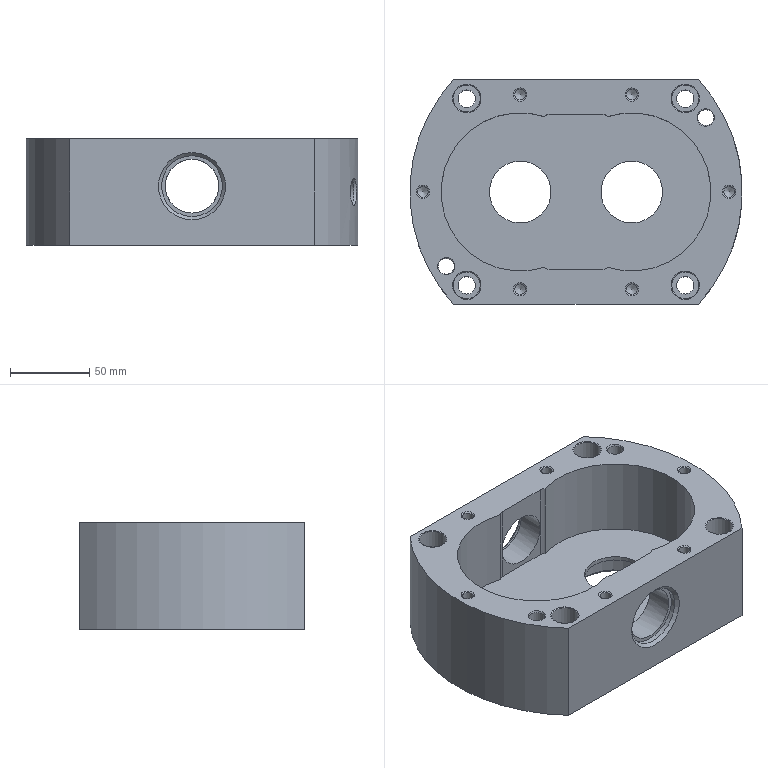NC program | NX | posted with a generic post | part box 210 x 142 x 67.4 mm
Lines 5220 to 5617 of 83330:
(FLOOR_WALL_2 , TOOL : D10JING)
N10396 T11 M6
N10398 G54
N10400 G17 G0 G90 X-51.734 Y60.143 B0. C0. S5000 M3
N10402 G43 Z30. H11
N10404 Z-1.
N10406 G94 G1 Z-2. F1000.
N10408 G3 X-52.5 Y60.5 R1.
N10410 G1 X52.5
N10412 Y50.048
N10414 G3 X52.804 Y49.589 R0.5
N10416 G1 X55.843 Y48.293
N10418 G2 X64.72 Y43.448 R52.5
N10420 G1 X65.991 Y42.586
N10422 G3 X66.272 Y42.5 R0.5
N10424 G1 X84.404
N10426 G2 X88.736 Y-32.5 R94.5
N10428 G1 X76.786
N10430 G3 X76.54 Y-32.564 R0.5
N10432 G1 X74.087 Y-28.207
N10434 G3 X65.035 Y37.641 R48.
N10436 X66.272 Y37.5 R5.5
N10438 G1 X81.265
N10440 G2 X83.739 Y31.591 R89.5
N10442 G1 X79.061 Y29.826
N10444 G3 X77.116 Y32.5 R53.
N10446 G1 X78.
N10448 G2 X79.061 Y29.826 R84.5
N10450 G1 X83.739 Y31.591
N10452 G2 X85.17 Y-27.5 R89.5
N10454 G1 X76.786
N10456 G3 X74.087 Y-28.207 R5.5
N10458 G1 X76.54 Y-32.564
N10460 X76.45 Y-32.589
N10462 X76.408 Y-32.672
N10464 X74.913 Y-34.397
N10466 G2 X55.843 Y-48.293 R52.5
N10468 G1 X52.804 Y-49.589
N10470 G3 X52.5 Y-50.048 R0.5
N10472 G1 Y-60.5
N10474 X-52.5
N10476 Y-50.048
N10478 G3 X-52.677 Y-49.667 R0.5
N10480 G1 X-49.443 Y-45.854
N10482 G3 X-2.402 Y-35. R48.
N10484 G1 X2.402
N10486 G3 X49.443 Y-45.854 R48.
N10488 X47.5 Y-50.048 R5.5
N10490 G1 Y-55.5
N10492 X-19.164
N10494 Y-50.5
N10496 G3 X-0.479 Y-40. R53.
N10498 G1 X0.479
N10500 G3 X19.164 Y-50.5 R53.
N10502 G1 X-0.75
N10504 Y-46.
N10506 G3 X0. Y-45.428 R57.5
N10508 X0.75 Y-46. R57.5
N10510 G1 X-0.75
N10512 Y-50.5
N10514 X-19.164
N10516 Y-55.5
N10518 X-47.5
N10520 Y-50.048
N10522 G3 X-49.443 Y-45.854 R5.5
N10524 G1 X-52.677 Y-49.667
N10526 X-52.804 Y-49.589
N10528 X-55.843 Y-48.293
N10530 G2 X-64.72 Y-43.448 R52.5
N10532 G1 X-65.991 Y-42.586
N10534 G3 X-66.272 Y-42.5 R0.5
N10536 G1 X-84.404
N10538 G2 X-88.736 Y32.5 R94.5
N10540 G1 X-76.786
N10542 G3 X-76.54 Y32.564 R0.5
N10544 G1 X-74.087 Y28.207
N10546 G3 X-65.035 Y-37.641 R48.
N10548 X-66.272 Y-37.5 R5.5
N10550 G1 X-81.265
N10552 G2 X-83.739 Y-31.591 R89.5
N10554 G1 X-79.061 Y-29.826
N10556 G3 X-77.116 Y-32.5 R53.
N10558 G1 X-78.
N10560 G2 X-79.061 Y-29.826 R84.5
N10562 G1 X-83.739 Y-31.591
N10564 G2 X-85.17 Y27.5 R89.5
N10566 G1 X-76.786
N10568 G3 X-74.087 Y28.207 R5.5
N10570 G1 X-76.54 Y32.564
N10572 X-76.45 Y32.589
N10574 X-76.408 Y32.672
N10576 X-74.913 Y34.397
N10578 G2 X-55.843 Y48.293 R52.5
N10580 G1 X-52.804 Y49.589
N10582 G3 X-52.5 Y50.048 R0.5
N10584 G1 Y60.5
N10586 X-47.5 Y55.5
N10588 X47.5
N10590 Y50.048
N10592 G3 X49.443 Y45.854 R5.5
N10594 X2.402 Y35. R48.
N10596 G1 X-2.402
N10598 G3 X-20.682 Y45.736 R48.
N10600 G1 X-19.164 Y50.5
N10602 X19.164
N10604 G3 X0.479 Y40. R53.
N10606 G1 X-0.479
N10608 G3 X-3.45 Y42.4 R53.
N10610 G1 X-0.75 Y46.
N10612 X0.75
N10614 G3 X0. Y45.428 R57.5
N10616 X-0.75 Y46. R57.5
N10618 G1 X-3.45 Y42.4
N10620 G3 X-19.164 Y50.5 R53.
N10622 G1 X-20.682 Y45.736
N10624 G3 X-49.443 Y45.854 R48.
N10626 G1 X-49.147 Y44.898
N10628 G2 X-2.8 Y34. R47.
N10630 G1 X2.8
N10632 G2 X2.8 Y-34. R-47.
N10634 G1 X-2.8
N10636 G2 X-49.147 Y44.898 R-47.
N10638 G1 X-49.443 Y45.854
N10640 G3 X-47.5 Y50.048 R5.5
N10642 G1 Y55.5
N10644 G3 X-47.857 Y56.266 R1.
N10646 G1 Z-1.
N10648 G0 Z30.
N10650 X-1.725 Y35.
N10652 Z-1.
N10654 G1 Z-2.
N10656 X-0.766 Y33.857
N10658 G3 X0. Y33.5 R1.
N10660 G1 X3.001
N10662 G2 X3.001 Y-33.5 R-46.5
N10664 G1 X-3.001
N10666 G2 X-3.001 Y33.5 R-46.5
N10668 G1 X0.
N10670 G3 X0.766 Y33.857 R1.
N10672 G1 X1.725 Y35.
N10674 Z-1.
N10676 G0 Z30.
N10678 Y59.5
N10680 Z-1.
N10682 G1 Z-2.
N10684 X0.766 Y60.643
N10686 G3 X0. Y61. R1.
N10688 G1 X-53.
N10690 Y50.048
N10692 X-56.039 Y48.753
N10694 G3 X-75.29 Y34.724 R53.
N10696 G1 X-76.786 Y33.
N10698 X-89.084
N10700 G3 X-84.711 Y-43. R95.
N10702 G1 X-66.272
N10704 X-65.001 Y-43.862
N10706 G3 X-56.039 Y-48.753 R53.
N10708 G1 X-53. Y-50.048
N10710 Y-61.
N10712 X53.
N10714 Y-50.048
N10716 X56.039 Y-48.753
N10718 G3 X75.29 Y-34.724 R53.
N10720 G1 X76.786 Y-33.
N10722 X89.084
N10724 G3 X84.711 Y43. R95.
N10726 G1 X66.272
N10728 X65.001 Y43.862
N10730 G3 X56.039 Y48.753 R53.
N10732 G1 X53. Y50.048
N10734 Y61.
N10736 X0.
N10738 G3 X-0.766 Y60.643 R1.
N10740 G1 X-1.305 Y60.
N10742 Z-1.
N10744 G0 Z30.
N10746 X68.5 Y-58.945
N10748 Z-0.9
N10750 G1 Y-59.176 Z-0.962
N10752 X68.824 Y-59.5 Z-1.085
N10754 X69. Z-1.132
N10756 X69.176 Z-1.179
N10758 X69.5 Y-59.176 Z-1.302
N10760 Y-59. Z-1.349
N10762 Y-58.824 Z-1.396
N10764 X69.176 Y-58.5 Z-1.519
N10766 X69. Z-1.566
N10768 X68.824 Z-1.613
N10770 X68.5 Y-58.824 Z-1.736
N10772 Y-59. Z-1.783
N10774 Y-59.176 Z-1.83
N10776 X68.824 Y-59.5 Z-1.953
N10778 X69. Z-2.
N10780 G3 X69.5 Y-59. R0.5
N10782 X69. Y-59.5 R-0.5
N10784 X69.383 Y-59.321 R0.5
N10786 G1 Z-1.
N10788 G0 Z30.
N10790 X51.734 Y-60.143
N10792 Z-6.
N10794 G1 Z-7.
N10796 G3 X52.5 Y-60.5 R1.
N10798 G1 X10.5
N10800 Y-55.
N10802 G3 X10. Y-54.5 R0.5
N10804 G1 X-10.
N10806 G3 X-10.5 Y-55. R0.5
N10808 G1 Y-60.5
N10810 X-52.5
N10812 Y-47.388
N10814 G3 X-52.795 Y-46.932 R0.5
N10816 G1 X-55.745 Y-45.606
N10818 G2 X-60.35 Y-43.243 R50.
N10820 G1 X-61.514 Y-42.568
N10822 G3 X-61.765 Y-42.5 R0.5
N10824 G1 X-84.404
N10826 G2 X-93.798 Y-11.5 R94.5
N10828 G1 X-82.367
N10830 G3 X-69.841 Y-33.995 R48.5
N10832 G1 X-73.408 Y-37.5
N10834 X-81.265
N10836 G2 X-87.966 Y-16.5 R89.5
N10838 G1 X-86.142
N10840 G3 X-73.408 Y-37.5 R53.5
N10842 G1 X-69.841 Y-33.995
N10844 G3 X-2.205 Y-35.5 R48.5
N10846 G1 X2.205
N10848 G3 X2.205 Y35.5 R-48.5
N10850 G1 X-2.205
N10852 G3 X-82.367 Y11.5 R48.5
N10854 G1 X-93.798
N10856 G2 X-88.736 Y32.5 R94.5
N10858 G1 X-81.141
N10860 Y27.5
N10862 G3 X-86.142 Y16.5 R53.5
N10864 G1 X-87.966
N10866 G2 X-85.17 Y27.5 R89.5
N10868 G1 X-81.141
N10870 Y32.5
N10872 X-73.537
N10874 G3 X-73.173 Y32.658 R0.5
N10876 G1 X-71.692 Y34.234
N10878 G2 X-55.745 Y45.606 R50.
N10880 G1 X-52.748 Y46.956
N10882 G3 X-52.5 Y47.388 R0.5
N10884 G1 Y60.5
N10886 X-10.5
N10888 Y55.
N10890 G3 X-10. Y54.5 R0.5
N10892 G1 X10.
N10894 G3 X10.5 Y55. R0.5
N10896 G1 Y60.5
N10898 X52.5
N10900 Y52.079
N10902 X47.5
N10904 G3 X0.293 Y40.5 R53.5
N10906 G1 X-0.293
N10908 G3 X-47.5 Y52.079 R53.5
N10910 G1 Y55.5
N10912 X-15.5
N10914 Y55.
N10916 G3 X-10. Y49.5 R5.5
N10918 G1 X10.
N10920 G3 X15.5 Y55. R5.5
N10922 G1 Y55.5
N10924 X47.5
N10926 Y52.079
N10928 X52.5
N10930 Y47.388
N10932 G3 X52.795 Y46.932 R0.5
N10934 G1 X55.745 Y45.606
N10936 G2 X60.35 Y43.243 R50.
N10938 G1 X61.524 Y42.562
N10940 G3 X61.765 Y42.5 R0.5
N10942 G1 X84.404
N10944 G2 X93.798 Y11.5 R94.5
N10946 G1 X87.966
N10948 X86.355
N10950 X86.144 Y16.495
N10952 G3 X73.408 Y37.5 R53.5
N10954 G1 X81.265
N10956 G2 X87.966 Y16.5 R89.5
N10958 G1 X86.376
N10960 G3 X86.144 Y16.495 R5.5
N10962 G1 X86.355 Y11.5
N10964 G3 X85.879 Y10.947 R0.5
N10966 G1 X86.464 Y5.421
N10968 G2 X86.464 Y-5.421 R51.5
N10970 G1 X85.879 Y-10.947
N10972 G3 X86.376 Y-11.5 R0.5
N10974 G1 X93.798
N10976 G2 X88.736 Y-32.5 R94.5
N10978 G1 X81.141
N10980 Y-27.5
N10982 G3 X86.144 Y-16.495 R53.5
N10984 X86.376 Y-16.5 R5.5
N10986 G1 X87.966
N10988 G2 X85.17 Y-27.5 R89.5
N10990 G1 X81.141
N10992 Y-32.5
N10994 X73.537
N10996 G3 X73.173 Y-32.658 R0.5
N10998 G1 X71.692 Y-34.234
N11000 G2 X55.745 Y-45.606 R50.
N11002 G1 X52.795 Y-46.932
N11004 G3 X52.5 Y-47.388 R0.5
N11006 G1 Y-60.5
N11008 X47.5 Y-55.5
N11010 X15.5
N11012 Y-55.
N11014 G3 X10. Y-49.5 R5.5
N11016 G1 X-10.
N11018 G3 X-15.5 Y-55. R5.5
N11020 G1 Y-55.5
N11022 X-47.5
N11024 Y-52.079
N11026 G3 X-0.293 Y-40.5 R53.5
N11028 G1 X0.293
N11030 G3 X47.5 Y-52.079 R53.5
N11032 G1 Y-55.5
N11034 X52.643 Y-56.266
N11036 G3 X53. Y-55.5 R1.
N11038 G1 Y-47.388
N11040 X55.95 Y-46.062
N11042 G3 X72.056 Y-34.577 R50.5
N11044 G1 X73.537 Y-33.
N11046 X89.084
N11048 G3 X94.361 Y-11. R95.
N11050 G1 X86.376
N11052 X86.961 Y-5.474
N11054 G3 X86.961 Y5.474 R52.
N11056 G1 X86.376 Y11.
N11058 X94.361
N11060 G3 X84.711 Y43. R95.
N11062 G1 X61.765
N11064 X60.601 Y43.676
N11066 G3 X55.95 Y46.062 R50.5
N11068 G1 X53. Y47.388
N11070 Y61.
N11072 X10.
N11074 Y55.
N11076 X-10.
N11078 Y61.
N11080 X-53.
N11082 Y47.388
N11084 X-55.95 Y46.062
N11086 G3 X-72.056 Y34.577 R50.5
N11088 G1 X-73.537 Y33.
N11090 X-89.084
N11092 G3 X-94.361 Y11. R95.
N11094 G1 X-81.973
N11096 G2 X-2.402 Y35. R48.
N11098 G1 X2.402
N11100 G2 X2.402 Y-35. R-48.
N11102 G1 X-2.402
N11104 G2 X-81.973 Y-11. R48.
N11106 G1 X-94.361
N11108 G3 X-84.711 Y-43. R95.
N11110 G1 X-61.765
N11112 X-60.601 Y-43.676
N11114 G3 X-55.95 Y-46.062 R50.5
N11116 G1 X-53. Y-47.388
N11118 Y-61.
N11120 X-10.
N11122 Y-55.
N11124 X10.
N11126 Y-61.
N11128 X53.
N11130 Y-55.5
N11132 G3 X52.643 Y-54.734 R1.
N11134 G1 X52. Y-54.195
N11136 Z-6.
N11138 G0 Z30.
N11140 X68.5 Y-58.945
N11142 Z-5.9
N11144 G1 Y-59.176 Z-5.962
N11146 X68.824 Y-59.5 Z-6.085
N11148 X69. Z-6.132
N11150 X69.176 Z-6.179
N11152 X69.5 Y-59.176 Z-6.302
N11154 Y-59. Z-6.349
N11156 Y-58.824 Z-6.396
N11158 X69.176 Y-58.5 Z-6.519
N11160 X69. Z-6.566
N11162 X68.824 Z-6.613
N11164 X68.5 Y-58.824 Z-6.736
N11166 Y-59. Z-6.783
N11168 Y-59.176 Z-6.83
N11170 X68.824 Y-59.5 Z-6.953
N11172 X69. Z-7.
N11174 G3 X69.5 Y-59. R0.5
N11176 X69. Y-59.5 R-0.5
N11178 X69.383 Y-59.321 R0.5
N11180 G1 Z-6.
N11182 G0 Z30.
N11184 M5